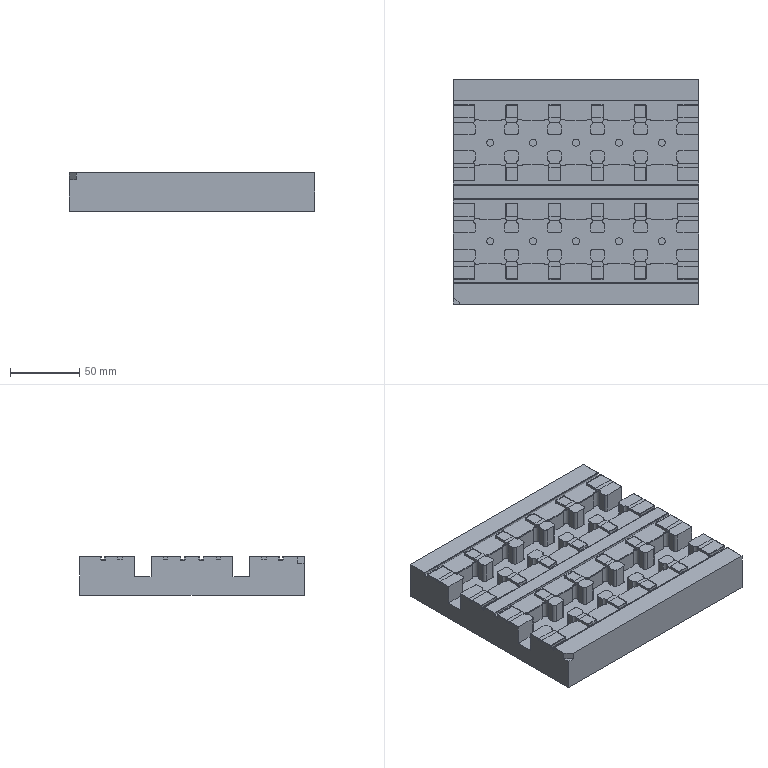NC program | NX | posted by the shop | part box 177 x 162 x 28 mm
Lines 35762 to 36755 of 254847:
N5 T05 M06
(D4  D=4. R=0. H=05 ce=0.02 di=0.05)
(D.N=05 MAX_Z=45. MIN_Z=13.55 Time=46.03M)
T04
G00 G90 G54 X69.164 Y47.661 M03 S4000
G43 H05 Z43.
M08
Z28.502
G01 X69.175 Z28.404 F1200.
X69.205 Y47.665 Z28.317
X69.253 Y47.673 Z28.241
X69.318 Y47.69 Z28.173
X69.396 Y47.717 Z28.114
X69.487 Y47.756 Z28.064
X69.589 Y47.811 Z28.022
X69.699 Y47.883 Z27.987
X69.816 Y47.975 Z27.959
X69.938 Y48.09 Z27.937
X70.063 Y48.229 Z27.921
X70.189 Y48.396 Z27.91
X70.314 Y48.593 Z27.904
X70.437 Y48.822 Z27.902
G02 X71.571 Y49.834 I1.813 J-.891 F1500.
G03 X71.757 Y50.097 I-.094 J.264
X71.663 Y50.307 I-.28 J0.0
G02 X70.986 Y51.668 I1.337 J1.514
G01 X70.965 Y51.832
X70.931 Y51.96 Z27.901
X70.886 Y52.051 Z27.9
X70.83 Y52.11 Z27.899
X70.767 Y52.139 Z27.897
X70.696 Y52.138 Z27.895
X70.62 Y52.112 Z27.893
X70.54 Y52.061 Z27.89
X70.457 Y51.988 Z27.888
X70.374 Y51.896 Z27.885
X70.291 Y51.786 Z27.882
X70.21 Y51.661 Z27.879
X70.132 Y51.523 Z27.875
X70.002 Y51.239 Z27.869
X69.891 Y50.928 Z27.863
X69.801 Y50.597 Z27.856
X69.734 Y50.258 Z27.849
X69.693 Y49.918 Z27.843
X69.678 Y49.588 Z27.837
X69.693 Y49.276 Z27.83
X69.713 Y49.119 Z27.827
X69.742 Y48.973 Z27.824
X69.778 Y48.84 Z27.821
X69.822 Y48.723 Z27.818
X69.872 Y48.625 Z27.815
X69.928 Y48.548 Z27.813
X69.99 Y48.494 Z27.811
X70.056 Y48.467 Z27.809
X70.127 Y48.47 Z27.807
X70.201 Y48.504 Z27.806
X70.277 Y48.572 Z27.805
X70.356 Y48.677 Z27.804
X70.437 Y48.822
G02 X71.571 Y49.834 I1.813 J-.891
G03 X71.757 Y50.097 I-.094 J.264
X71.663 Y50.307 I-.28 J0.0
G02 X70.986 Y51.668 I1.337 J1.514
G01 X70.965 Y51.832 Z27.803
X70.931 Y51.96
X70.886 Y52.051 Z27.802
X70.83 Y52.11 Z27.801
X70.767 Y52.139 Z27.799
X70.696 Y52.138 Z27.797
X70.62 Y52.112 Z27.795
X70.54 Y52.061 Z27.792
X70.457 Y51.988 Z27.789
X70.374 Y51.896 Z27.787
X70.291 Y51.786 Z27.784
X70.21 Y51.661 Z27.78
X70.132 Y51.523 Z27.777
X70.002 Y51.239 Z27.771
X69.891 Y50.928 Z27.764
X69.801 Y50.597 Z27.758
X69.734 Y50.258 Z27.751
X69.693 Y49.918 Z27.745
X69.678 Y49.588 Z27.738
X69.693 Y49.276 Z27.732
X69.713 Y49.119 Z27.729
X69.742 Y48.973 Z27.726
X69.778 Y48.84 Z27.723
X69.822 Y48.723 Z27.72
X69.872 Y48.625 Z27.717
X69.928 Y48.548 Z27.715
X69.99 Y48.494 Z27.712
X70.056 Y48.467 Z27.71
X70.127 Y48.47 Z27.709
X70.201 Y48.504 Z27.707
X70.277 Y48.572 Z27.706
X70.356 Y48.677
X70.437 Y48.822
G02 X71.571 Y49.834 I1.813 J-.891
G03 X71.757 Y50.097 I-.094 J.264
X71.663 Y50.307 I-.28 J0.0
G02 X70.986 Y51.668 I1.337 J1.514
G01 X70.965 Y51.832 Z27.705
X70.931 Y51.96
X70.886 Y52.051 Z27.704
X70.83 Y52.11 Z27.702
X70.767 Y52.139 Z27.701
X70.696 Y52.138 Z27.699
X70.62 Y52.112 Z27.696
X70.54 Y52.061 Z27.694
X70.457 Y51.988 Z27.691
X70.374 Y51.896 Z27.688
X70.291 Y51.786 Z27.685
X70.21 Y51.661 Z27.682
X70.132 Y51.523 Z27.679
X70.002 Y51.239 Z27.673
X69.891 Y50.928 Z27.666
X69.801 Y50.597 Z27.66
X69.734 Y50.258 Z27.653
X69.693 Y49.918 Z27.647
X69.678 Y49.588 Z27.64
X69.693 Y49.276 Z27.634
X69.713 Y49.119 Z27.631
X69.742 Y48.973 Z27.628
X69.778 Y48.84 Z27.625
X69.822 Y48.723 Z27.622
X69.872 Y48.625 Z27.619
X69.928 Y48.548 Z27.616
X69.99 Y48.494 Z27.614
X70.056 Y48.467 Z27.612
X70.127 Y48.47 Z27.611
X70.201 Y48.504 Z27.609
X70.277 Y48.572 Z27.608
X70.356 Y48.677
X70.437 Y48.822 Z27.607
G02 X71.571 Y49.834 I1.813 J-.891
G03 X71.757 Y50.097 I-.094 J.264
X71.663 Y50.307 I-.28 J0.0
G02 X70.986 Y51.668 I1.337 J1.514
G01 X70.965 Y51.832
X70.931 Y51.96
X70.886 Y52.051 Z27.606
X70.83 Y52.11 Z27.604
X70.767 Y52.139 Z27.603
X70.696 Y52.138 Z27.601
X70.62 Y52.112 Z27.598
X70.54 Y52.061 Z27.596
X70.457 Y51.988 Z27.593
X70.374 Y51.896 Z27.59
X70.291 Y51.786 Z27.587
X70.21 Y51.661 Z27.584
X70.132 Y51.523 Z27.581
X70.002 Y51.239 Z27.575
X69.891 Y50.928 Z27.568
X69.801 Y50.597 Z27.562
X69.734 Y50.258 Z27.555
X69.693 Y49.918 Z27.549
X69.678 Y49.588 Z27.542
X69.693 Y49.276 Z27.536
X69.713 Y49.119 Z27.533
X69.742 Y48.973 Z27.529
X69.778 Y48.84 Z27.526
X69.822 Y48.723 Z27.524
X69.872 Y48.625 Z27.521
X69.928 Y48.548 Z27.518
X69.99 Y48.494 Z27.516
X70.056 Y48.467 Z27.514
X70.127 Y48.47 Z27.512
X70.201 Y48.504 Z27.511
X70.277 Y48.572 Z27.51
X70.356 Y48.677 Z27.509
X70.437 Y48.822
G02 X71.571 Y49.834 I1.813 J-.891
G03 X71.757 Y50.097 I-.094 J.264
X71.663 Y50.307 I-.28 J0.0
G02 X70.986 Y51.668 I1.337 J1.514
G01 X70.965 Y51.832
X70.931 Y51.96 Z27.508
X70.886 Y52.051 Z27.507
X70.83 Y52.11 Z27.506
X70.767 Y52.139 Z27.504
X70.696 Y52.138 Z27.502
X70.62 Y52.112 Z27.5
X70.54 Y52.061 Z27.498
X70.457 Y51.988 Z27.495
X70.374 Y51.896 Z27.492
X70.291 Y51.786 Z27.489
X70.21 Y51.661 Z27.486
X70.132 Y51.523 Z27.483
X70.002 Y51.239 Z27.476
X69.891 Y50.928 Z27.47
X69.801 Y50.597 Z27.463
X69.734 Y50.258 Z27.457
X69.693 Y49.918 Z27.45
X69.678 Y49.588 Z27.444
X69.693 Y49.276 Z27.438
X69.713 Y49.119 Z27.434
X69.742 Y48.973 Z27.431
X69.778 Y48.84 Z27.428
X69.822 Y48.723 Z27.425
X69.872 Y48.625 Z27.423
X69.928 Y48.548 Z27.42
X69.99 Y48.494 Z27.418
X70.056 Y48.467 Z27.416
X70.127 Y48.47 Z27.414
X70.201 Y48.504 Z27.413
X70.277 Y48.572 Z27.412
X70.356 Y48.677 Z27.411
X70.437 Y48.822
G02 X71.571 Y49.834 I1.813 J-.891
G03 X71.757 Y50.097 I-.094 J.264
X71.663 Y50.307 I-.28 J0.0
G02 X70.986 Y51.668 I1.337 J1.514
G01 X70.965 Y51.832
X70.931 Y51.96 Z27.41
X70.886 Y52.051 Z27.409
X70.83 Y52.11 Z27.408
X70.767 Y52.139 Z27.406
X70.696 Y52.138 Z27.404
X70.62 Y52.112 Z27.402
X70.54 Y52.061 Z27.4
X70.457 Y51.988 Z27.397
X70.374 Y51.896 Z27.394
X70.291 Y51.786 Z27.391
X70.21 Y51.661 Z27.388
X70.132 Y51.523 Z27.385
X70.002 Y51.239 Z27.378
X69.891 Y50.928 Z27.372
X69.801 Y50.597 Z27.365
X69.734 Y50.258 Z27.359
X69.693 Y49.918 Z27.352
X69.678 Y49.588 Z27.346
X69.693 Y49.276 Z27.34
X69.713 Y49.119 Z27.336
X69.742 Y48.973 Z27.333
X69.778 Y48.84 Z27.33
X69.822 Y48.723 Z27.327
X69.872 Y48.625 Z27.325
X69.928 Y48.548 Z27.322
X69.99 Y48.494 Z27.32
X70.056 Y48.467 Z27.318
X70.127 Y48.47 Z27.316
X70.201 Y48.504 Z27.315
X70.277 Y48.572 Z27.314
X70.356 Y48.677 Z27.313
X70.437 Y48.822
G02 X71.571 Y49.834 I1.813 J-.891
G03 X71.757 Y50.097 I-.094 J.264
X71.663 Y50.307 I-.28 J0.0
G02 X70.986 Y51.668 I1.337 J1.514
G01 X70.965 Y51.832
X70.931 Y51.96 Z27.312
X70.886 Y52.051 Z27.311
X70.83 Y52.11 Z27.31
X70.767 Y52.139 Z27.308
X70.696 Y52.138 Z27.306
X70.62 Y52.112 Z27.304
X70.54 Y52.061 Z27.301
X70.457 Y51.988 Z27.299
X70.374 Y51.896 Z27.296
X70.291 Y51.786 Z27.293
X70.21 Y51.661 Z27.29
X70.132 Y51.523 Z27.286
X70.002 Y51.239 Z27.28
X69.891 Y50.928 Z27.274
X69.801 Y50.597 Z27.267
X69.734 Y50.258 Z27.261
X69.693 Y49.918 Z27.254
X69.678 Y49.588 Z27.248
X69.693 Y49.276 Z27.241
X69.713 Y49.119 Z27.238
X69.742 Y48.973 Z27.235
X69.778 Y48.84 Z27.232
X69.822 Y48.723 Z27.229
X69.872 Y48.625 Z27.226
X69.928 Y48.548 Z27.224
X69.99 Y48.494 Z27.222
X70.056 Y48.467 Z27.22
X70.127 Y48.47 Z27.218
X70.201 Y48.504 Z27.217
X70.277 Y48.572 Z27.216
X70.356 Y48.677 Z27.215
X70.437 Y48.822
G02 X71.571 Y49.834 I1.813 J-.891
G03 X71.757 Y50.097 I-.094 J.264
X71.663 Y50.307 I-.28 J0.0
G02 X70.986 Y51.668 I1.337 J1.514
G01 X70.965 Y51.832
X70.931 Y51.96 Z27.214
X70.886 Y52.051 Z27.213
X70.83 Y52.11 Z27.212
X70.767 Y52.139 Z27.21
X70.696 Y52.138 Z27.208
X70.62 Y52.112 Z27.206
X70.54 Y52.061 Z27.203
X70.457 Y51.988 Z27.201
X70.374 Y51.896 Z27.198
X70.291 Y51.786 Z27.195
X70.21 Y51.661 Z27.191
X70.132 Y51.523 Z27.188
X70.002 Y51.239 Z27.182
X69.891 Y50.928 Z27.176
X69.801 Y50.597 Z27.169
X69.734 Y50.258 Z27.162
X69.693 Y49.918 Z27.156
X69.678 Y49.588 Z27.149
X69.693 Y49.276 Z27.143
X69.713 Y49.119 Z27.14
X69.742 Y48.973 Z27.137
X69.778 Y48.84 Z27.134
X69.822 Y48.723 Z27.131
X69.872 Y48.625 Z27.128
X69.928 Y48.548 Z27.126
X69.99 Y48.494 Z27.124
X70.056 Y48.467 Z27.122
X70.127 Y48.47 Z27.12
X70.201 Y48.504 Z27.119
X70.277 Y48.572 Z27.118
X70.356 Y48.677 Z27.117
X70.437 Y48.822
G02 X71.571 Y49.834 I1.813 J-.891
G03 X71.757 Y50.097 I-.094 J.264
X71.663 Y50.307 I-.28 J0.0
G02 X70.986 Y51.668 I1.337 J1.514
G01 X70.965 Y51.832 Z27.116
X70.931 Y51.96
X70.886 Y52.051 Z27.115
X70.83 Y52.11 Z27.113
X70.767 Y52.139 Z27.112
X70.696 Y52.138 Z27.11
X70.62 Y52.112 Z27.108
X70.54 Y52.061 Z27.105
X70.457 Y51.988 Z27.102
X70.374 Y51.896 Z27.1
X70.291 Y51.786 Z27.097
X70.21 Y51.661 Z27.093
X70.132 Y51.523 Z27.09
X70.002 Y51.239 Z27.084
X69.891 Y50.928 Z27.077
X69.801 Y50.597 Z27.071
X69.734 Y50.258 Z27.064
X69.693 Y49.918 Z27.058
X69.678 Y49.588 Z27.051
X69.693 Y49.276 Z27.045
X69.713 Y49.119 Z27.042
X69.742 Y48.973 Z27.039
X69.778 Y48.84 Z27.036
X69.822 Y48.723 Z27.033
X69.872 Y48.625 Z27.03
X69.928 Y48.548 Z27.028
X69.99 Y48.494 Z27.025
X70.056 Y48.467 Z27.023
X70.127 Y48.47 Z27.022
X70.201 Y48.504 Z27.02
X70.277 Y48.572 Z27.019
X70.356 Y48.677
X70.437 Y48.822
G02 X71.571 Y49.834 I1.813 J-.891
G03 X71.757 Y50.097 I-.094 J.264
X71.663 Y50.307 I-.28 J0.0
G02 X70.986 Y51.668 I1.337 J1.514
G01 X70.965 Y51.832 Z27.018
X70.931 Y51.96
X70.886 Y52.051 Z27.017
X70.83 Y52.11 Z27.015
X70.767 Y52.139 Z27.014
X70.696 Y52.138 Z27.012
X70.62 Y52.112 Z27.009
X70.54 Y52.061 Z27.007
X70.457 Y51.988 Z27.004
X70.374 Y51.896 Z27.001
X70.291 Y51.786 Z26.998
X70.21 Y51.661 Z26.995
X70.132 Y51.523 Z26.992
X70.002 Y51.239 Z26.986
X69.891 Y50.928 Z26.979
X69.801 Y50.597 Z26.973
X69.734 Y50.258 Z26.966
X69.693 Y49.918 Z26.96
X69.678 Y49.588 Z26.953
X69.693 Y49.276 Z26.947
X69.713 Y49.119 Z26.944
X69.742 Y48.973 Z26.941
X69.778 Y48.84 Z26.937
X69.822 Y48.723 Z26.935
X69.872 Y48.625 Z26.932
X69.928 Y48.548 Z26.929
X69.99 Y48.494 Z26.927
X70.056 Y48.467 Z26.925
X70.127 Y48.47 Z26.924
X70.201 Y48.504 Z26.922
X70.277 Y48.572 Z26.921
X70.356 Y48.677
X70.437 Y48.822 Z26.92
G02 X71.571 Y49.834 I1.813 J-.891
G03 X71.757 Y50.097 I-.094 J.264
X71.663 Y50.307 I-.28 J0.0
G02 X70.986 Y51.668 I1.337 J1.514
G01 X70.965 Y51.832
X70.931 Y51.96
X70.886 Y52.051 Z26.919
X70.83 Y52.11 Z26.917
X70.767 Y52.139 Z26.916
X70.696 Y52.138 Z26.914
X70.62 Y52.112 Z26.911
X70.54 Y52.061 Z26.909
X70.457 Y51.988 Z26.906
X70.374 Y51.896 Z26.903
X70.291 Y51.786 Z26.9
X70.21 Y51.661 Z26.897
X70.132 Y51.523 Z26.894
X70.002 Y51.239 Z26.888
X69.891 Y50.928 Z26.881
X69.801 Y50.597 Z26.875
X69.734 Y50.258 Z26.868
X69.693 Y49.918 Z26.861
X69.678 Y49.588 Z26.855
X69.693 Y49.276 Z26.849
X69.713 Y49.119 Z26.846
X69.742 Y48.973 Z26.842
X69.778 Y48.84 Z26.839
X69.822 Y48.723 Z26.836
X69.872 Y48.625 Z26.834
X69.928 Y48.548 Z26.831
X69.99 Y48.494 Z26.829
X70.056 Y48.467 Z26.827
X70.127 Y48.47 Z26.825
X70.201 Y48.504 Z26.824
X70.277 Y48.572 Z26.823
X70.356 Y48.677 Z26.822
X70.437 Y48.822
G02 X71.571 Y49.834 I1.813 J-.891
G03 X71.757 Y50.097 I-.094 J.264
X71.663 Y50.307 I-.28 J0.0
G02 X70.986 Y51.668 I1.337 J1.514
G01 X70.965 Y51.832
X70.931 Y51.96 Z26.821
X70.886 Y52.051 Z26.82
X70.83 Y52.11 Z26.819
X70.767 Y52.139 Z26.817
X70.696 Y52.138 Z26.815
X70.62 Y52.112 Z26.813
X70.54 Y52.061 Z26.811
X70.457 Y51.988 Z26.808
X70.374 Y51.896 Z26.805
X70.291 Y51.786 Z26.802
X70.21 Y51.661 Z26.799
X70.132 Y51.523 Z26.796
X70.002 Y51.239 Z26.789
X69.891 Y50.928 Z26.783
X69.801 Y50.597 Z26.776
X69.734 Y50.258 Z26.77
X69.693 Y49.918 Z26.763
X69.678 Y49.588 Z26.757
X69.693 Y49.276 Z26.751
X69.713 Y49.119 Z26.747
X69.742 Y48.973 Z26.744
X69.778 Y48.84 Z26.741
X69.822 Y48.723 Z26.738
X69.872 Y48.625 Z26.736
X69.928 Y48.548 Z26.733
X69.99 Y48.494 Z26.731
X70.056 Y48.467 Z26.729
X70.127 Y48.47 Z26.727
X70.201 Y48.504 Z26.726
X70.277 Y48.572 Z26.725
X70.356 Y48.677 Z26.724
X70.437 Y48.822
G02 X71.571 Y49.834 I1.813 J-.891
G03 X71.757 Y50.097 I-.094 J.264
X71.663 Y50.307 I-.28 J0.0
G02 X70.986 Y51.668 I1.337 J1.514
G01 X70.965 Y51.832
X70.931 Y51.96 Z26.723
X70.886 Y52.051 Z26.722
X70.83 Y52.11 Z26.721
X70.767 Y52.139 Z26.719
X70.696 Y52.138 Z26.717
X70.62 Y52.112 Z26.715
X70.54 Y52.061 Z26.713
X70.457 Y51.988 Z26.71
X70.374 Y51.896 Z26.707
X70.291 Y51.786 Z26.704
X70.21 Y51.661 Z26.701
X70.132 Y51.523 Z26.697
X70.002 Y51.239 Z26.691
X69.891 Y50.928 Z26.685
X69.801 Y50.597 Z26.678
X69.734 Y50.258 Z26.672
X69.693 Y49.918 Z26.665
X69.678 Y49.588 Z26.659
X69.693 Y49.276 Z26.653
X69.713 Y49.119 Z26.649
X69.742 Y48.973 Z26.646
X69.778 Y48.84 Z26.643
X69.822 Y48.723 Z26.64
X69.872 Y48.625 Z26.637
X69.928 Y48.548 Z26.635
X69.99 Y48.494 Z26.633
X70.056 Y48.467 Z26.631
X70.127 Y48.47 Z26.629
X70.201 Y48.504 Z26.628
X70.277 Y48.572 Z26.627
X70.356 Y48.677 Z26.626
X70.437 Y48.822
G02 X71.571 Y49.834 I1.813 J-.891
G03 X71.757 Y50.097 I-.094 J.264
X71.663 Y50.307 I-.28 J0.0
G02 X70.986 Y51.668 I1.337 J1.514
G01 X70.965 Y51.832
X70.931 Y51.96 Z26.625
X70.886 Y52.051 Z26.624
X70.83 Y52.11 Z26.623
X70.767 Y52.139 Z26.621
X70.696 Y52.138 Z26.619
X70.62 Y52.112 Z26.617
X70.54 Y52.061 Z26.614
X70.457 Y51.988 Z26.612
X70.374 Y51.896 Z26.609
X70.291 Y51.786 Z26.606
X70.21 Y51.661 Z26.603
X70.132 Y51.523 Z26.599
X70.002 Y51.239 Z26.593
X69.891 Y50.928 Z26.587
X69.801 Y50.597 Z26.58
X69.734 Y50.258 Z26.574
X69.693 Y49.918 Z26.567
X69.678 Y49.588 Z26.561
X69.693 Y49.276 Z26.554
X69.713 Y49.119 Z26.551
X69.742 Y48.973 Z26.548
X69.778 Y48.84 Z26.545
X69.822 Y48.723 Z26.542
X69.872 Y48.625 Z26.539
X69.928 Y48.548 Z26.537
X69.99 Y48.494 Z26.535
X70.056 Y48.467 Z26.533
X70.127 Y48.47 Z26.531
X70.201 Y48.504 Z26.53
X70.277 Y48.572 Z26.529
X70.356 Y48.677 Z26.528
X70.437 Y48.822
G02 X71.571 Y49.834 I1.813 J-.891
G03 X71.757 Y50.097 I-.094 J.264
X71.663 Y50.307 I-.28 J0.0
G02 X70.986 Y51.668 I1.337 J1.514
G01 X70.965 Y51.832
X70.931 Y51.96 Z26.527
X70.886 Y52.051 Z26.526
X70.83 Y52.11 Z26.525
X70.767 Y52.139 Z26.523
X70.696 Y52.138 Z26.521
X70.62 Y52.112 Z26.519
X70.54 Y52.061 Z26.516
X70.457 Y51.988 Z26.514
X70.374 Y51.896 Z26.511
X70.291 Y51.786 Z26.508
X70.21 Y51.661 Z26.504
X70.132 Y51.523 Z26.501
X70.002 Y51.239 Z26.495
X69.891 Y50.928 Z26.489
X69.801 Y50.597 Z26.482
X69.734 Y50.258 Z26.475
X69.693 Y49.918 Z26.469
X69.678 Y49.588 Z26.462
X69.693 Y49.276 Z26.456
X69.713 Y49.119 Z26.453
X69.742 Y48.973 Z26.45
X69.778 Y48.84 Z26.447
X69.822 Y48.723 Z26.444
X69.872 Y48.625 Z26.441
X69.928 Y48.548 Z26.439
X69.99 Y48.494 Z26.436
X70.056 Y48.467 Z26.434
X70.127 Y48.47 Z26.433
X70.201 Y48.504 Z26.431
X70.277 Y48.572 Z26.43
X70.356 Y48.677
X70.437 Y48.822
G02 X71.571 Y49.834 I1.813 J-.891
G03 X71.757 Y50.097 I-.094 J.264
X71.663 Y50.307 I-.28 J0.0
G02 X70.986 Y51.668 I1.337 J1.514
G01 X70.965 Y51.832 Z26.429
X70.931 Y51.96
X70.886 Y52.051 Z26.428
X70.83 Y52.11 Z26.426
X70.767 Y52.139 Z26.425
X70.696 Y52.138 Z26.423
X70.62 Y52.112 Z26.421
X70.54 Y52.061 Z26.418
X70.457 Y51.988 Z26.415
X70.374 Y51.896 Z26.413
X70.291 Y51.786 Z26.409
X70.21 Y51.661 Z26.406
X70.132 Y51.523 Z26.403
X70.002 Y51.239 Z26.397
X69.891 Y50.928 Z26.39
X69.801 Y50.597 Z26.384
X69.734 Y50.258 Z26.377
X69.693 Y49.918 Z26.371
X69.678 Y49.588 Z26.364
X69.693 Y49.276 Z26.358
X69.713 Y49.119 Z26.355
X69.742 Y48.973 Z26.352
X69.778 Y48.84 Z26.349
X69.822 Y48.723 Z26.346
X69.872 Y48.625 Z26.343
X69.928 Y48.548 Z26.341
X69.99 Y48.494 Z26.338
X70.056 Y48.467 Z26.336
X70.127 Y48.47 Z26.335
X70.201 Y48.504 Z26.333
X70.277 Y48.572 Z26.332
X70.356 Y48.677
X70.437 Y48.822 Z26.331
G02 X71.571 Y49.834 I1.813 J-.891
G03 X71.757 Y50.097 I-.094 J.264
X71.663 Y50.307 I-.28 J0.0
G02 X70.986 Y51.668 I1.337 J1.514
G01 X70.965 Y51.832
X70.931 Y51.96
X70.886 Y52.051 Z26.33
X70.83 Y52.11 Z26.328
X70.767 Y52.139 Z26.327
X70.696 Y52.138 Z26.325
X70.62 Y52.112 Z26.322
X70.54 Y52.061 Z26.32
X70.457 Y51.988 Z26.317
X70.374 Y51.896 Z26.314
X70.291 Y51.786 Z26.311
X70.21 Y51.661 Z26.308
X70.132 Y51.523 Z26.305
X70.002 Y51.239 Z26.299
X69.891 Y50.928 Z26.292
X69.801 Y50.597 Z26.286
X69.734 Y50.258 Z26.279
X69.693 Y49.918 Z26.273
X69.678 Y49.588 Z26.266
X69.693 Y49.276 Z26.26
X69.713 Y49.119 Z26.257
X69.742 Y48.973 Z26.253
X69.778 Y48.84 Z26.25
X69.822 Y48.723 Z26.248
X69.872 Y48.625 Z26.245
X69.928 Y48.548 Z26.242
X69.99 Y48.494 Z26.24
X70.056 Y48.467 Z26.238
X70.127 Y48.47 Z26.237
X70.201 Y48.504 Z26.235
X70.277 Y48.572 Z26.234
X70.356 Y48.677
X70.437 Y48.822 Z26.233
G02 X71.571 Y49.834 I1.813 J-.891
G03 X71.757 Y50.097 I-.094 J.264
X71.663 Y50.307 I-.28 J0.0
G02 X70.986 Y51.668 I1.337 J1.514
G01 X70.965 Y51.832
X70.931 Y51.96
X70.886 Y52.051 Z26.231
X70.83 Y52.11 Z26.23
X70.767 Y52.139 Z26.228
X70.696 Y52.138 Z26.226
X70.62 Y52.112 Z26.224
X70.54 Y52.061 Z26.222
X70.457 Y51.988 Z26.219
X70.374 Y51.896 Z26.216
X70.291 Y51.786 Z26.213
X70.21 Y51.661 Z26.21
X70.132 Y51.523 Z26.207
X70.002 Y51.239 Z26.201
X69.891 Y50.928 Z26.194
X69.801 Y50.597 Z26.188
X69.734 Y50.258 Z26.181
X69.693 Y49.918 Z26.174
X69.678 Y49.588 Z26.168
X69.693 Y49.276 Z26.162
X69.713 Y49.119 Z26.159
X69.742 Y48.973 Z26.155
X69.778 Y48.84 Z26.152
X69.822 Y48.723 Z26.149
X69.872 Y48.625 Z26.147
X69.928 Y48.548 Z26.144
X69.99 Y48.494 Z26.142
X70.056 Y48.467 Z26.14
X70.127 Y48.47 Z26.138
X70.201 Y48.504 Z26.137
X70.277 Y48.572 Z26.136
X70.356 Y48.677 Z26.135
X70.437 Y48.822
G02 X71.571 Y49.834 I1.813 J-.891
G03 X71.757 Y50.097 I-.094 J.264
X71.663 Y50.307 I-.28 J0.0
G02 X70.986 Y51.668 I1.337 J1.514
G01 X70.965 Y51.832
X70.931 Y51.96 Z26.134
X70.886 Y52.051 Z26.133
X70.83 Y52.11 Z26.132
X70.767 Y52.139 Z26.13
X70.696 Y52.138 Z26.128
X70.62 Y52.112 Z26.126
X70.54 Y52.061 Z26.124
X70.457 Y51.988 Z26.121
X70.374 Y51.896 Z26.118
X70.291 Y51.786 Z26.115
X70.21 Y51.661 Z26.112
X70.132 Y51.523 Z26.109
X70.002 Y51.239 Z26.102
X69.891 Y50.928 Z26.096
X69.801 Y50.597 Z26.089
X69.734 Y50.258 Z26.083
X69.693 Y49.918 Z26.076
X69.678 Y49.588 Z26.07
X69.693 Y49.276 Z26.064
X69.713 Y49.119 Z26.06
X69.742 Y48.973 Z26.057
X69.778 Y48.84 Z26.054
X69.822 Y48.723 Z26.051
X69.872 Y48.625 Z26.049
X69.928 Y48.548 Z26.046
X69.99 Y48.494 Z26.044
X70.056 Y48.467 Z26.042
X70.127 Y48.47 Z26.04
X70.201 Y48.504 Z26.039
X70.277 Y48.572 Z26.038
X70.356 Y48.677 Z26.037
X70.437 Y48.822
G02 X71.571 Y49.834 I1.813 J-.891
G03 X71.757 Y50.097 I-.094 J.264
X71.663 Y50.307 I-.28 J0.0
G02 X70.986 Y51.668 I1.337 J1.514
G01 X70.965 Y51.832
X70.931 Y51.96 Z26.036
X70.886 Y52.051 Z26.035
X70.83 Y52.11 Z26.034
X70.767 Y52.139 Z26.032
X70.696 Y52.138 Z26.03
X70.62 Y52.112 Z26.028
X70.54 Y52.061 Z26.025
X70.457 Y51.988 Z26.023
X70.374 Y51.896 Z26.02
X70.291 Y51.786 Z26.017
X70.21 Y51.661 Z26.014
X70.132 Y51.523 Z26.01
X70.002 Y51.239 Z26.004
X69.891 Y50.928 Z25.998
X69.801 Y50.597 Z25.991
X69.734 Y50.258 Z25.985
X69.693 Y49.918 Z25.978
X69.678 Y49.588 Z25.972
X69.693 Y49.276 Z25.965
X69.713 Y49.119 Z25.962
X69.742 Y48.973 Z25.959
X69.778 Y48.84 Z25.956
X69.822 Y48.723 Z25.953
X69.872 Y48.625 Z25.95
X69.928 Y48.548 Z25.948
X69.99 Y48.494 Z25.946
X70.056 Y48.467 Z25.944
X70.127 Y48.47 Z25.942
X70.201 Y48.504 Z25.941
X70.277 Y48.572 Z25.94
X70.356 Y48.677 Z25.939
X70.437 Y48.822
G02 X71.571 Y49.834 I1.813 J-.891
G03 X71.757 Y50.097 I-.094 J.264
X71.663 Y50.307 I-.28 J0.0
G02 X70.986 Y51.668 I1.337 J1.514
G01 X70.965 Y51.832
X70.931 Y51.96 Z25.938
X70.886 Y52.051 Z25.937
X70.83 Y52.11 Z25.936
X70.767 Y52.139 Z25.934
X70.696 Y52.138 Z25.932
X70.62 Y52.112 Z25.93
X70.54 Y52.061 Z25.927
X70.457 Y51.988 Z25.925
X70.374 Y51.896 Z25.922
X70.291 Y51.786 Z25.919
X70.21 Y51.661 Z25.916
X70.132 Y51.523 Z25.912
X70.002 Y51.239 Z25.906
X69.891 Y50.928 Z25.9
X69.801 Y50.597 Z25.893
X69.734 Y50.258 Z25.887
X69.693 Y49.918 Z25.88
X69.678 Y49.588 Z25.874
X69.693 Y49.276 Z25.867
X69.713 Y49.119 Z25.864
X69.742 Y48.973 Z25.861
X69.778 Y48.84 Z25.858
X69.822 Y48.723 Z25.855
X69.872 Y48.625 Z25.852
X69.928 Y48.548 Z25.85
X69.99 Y48.494 Z25.848
X70.056 Y48.467 Z25.846
X70.127 Y48.47 Z25.844
X70.201 Y48.504 Z25.843
X70.277 Y48.572 Z25.842
X70.356 Y48.677 Z25.841
X70.437 Y48.822
G02 X71.571 Y49.834 I1.813 J-.891
G03 X71.757 Y50.097 I-.094 J.264
X71.663 Y50.307 I-.28 J0.0
G02 X70.986 Y51.668 I1.337 J1.514
G01 X70.965 Y51.832
X70.931 Y51.96 Z25.84
X70.886 Y52.051 Z25.839
X70.83 Y52.11 Z25.838
X70.767 Y52.139 Z25.836
X70.696 Y52.138 Z25.834
X70.62 Y52.112 Z25.832
X70.54 Y52.061 Z25.829
X70.457 Y51.988 Z25.826
X70.374 Y51.896 Z25.824
X70.291 Y51.786 Z25.821
X70.21 Y51.661 Z25.817
X70.132 Y51.523 Z25.814
X70.002 Y51.239 Z25.808
X69.891 Y50.928 Z25.801
X69.801 Y50.597 Z25.795
X69.734 Y50.258 Z25.788
X69.693 Y49.918 Z25.782
X69.678 Y49.588 Z25.775
X69.693 Y49.276 Z25.769
X69.713 Y49.119 Z25.766
X69.742 Y48.973 Z25.763
X69.778 Y48.84 Z25.76
X69.822 Y48.723 Z25.757
X69.872 Y48.625 Z25.754
X69.928 Y48.548 Z25.752
X69.99 Y48.494 Z25.749
X70.056 Y48.467 Z25.747
X70.127 Y48.47 Z25.746
X70.201 Y48.504 Z25.744
X70.277 Y48.572 Z25.743
X70.356 Y48.677
X70.437 Y48.822
G02 X71.571 Y49.834 I1.813 J-.891
G03 X71.757 Y50.097 I-.094 J.264
X71.663 Y50.307 I-.28 J0.0
G02 X70.986 Y51.668 I1.337 J1.514
G01 X70.965 Y51.832 Z25.742
X70.931 Y51.96
X70.886 Y52.051 Z25.741
X70.83 Y52.11 Z25.739
X70.767 Y52.139 Z25.738
X70.696 Y52.138 Z25.736
X70.62 Y52.112 Z25.734
X70.54 Y52.061 Z25.731
X70.457 Y51.988 Z25.728
X70.374 Y51.896 Z25.725
X70.291 Y51.786 Z25.722
X70.21 Y51.661 Z25.719
X70.132 Y51.523 Z25.716
X70.002 Y51.239 Z25.71
X69.891 Y50.928 Z25.703
X69.801 Y50.597 Z25.697
X69.734 Y50.258 Z25.69
X69.693 Y49.918 Z25.684
X69.678 Y49.588 Z25.677
X69.693 Y49.276 Z25.671
X69.713 Y49.119 Z25.668
X69.742 Y48.973 Z25.665
X69.778 Y48.84 Z25.662
X69.822 Y48.723 Z25.659
X69.872 Y48.625 Z25.656
X69.928 Y48.548 Z25.654
X69.99 Y48.494 Z25.651
X70.056 Y48.467 Z25.649
X70.127 Y48.47 Z25.648
X70.201 Y48.504 Z25.646
X70.277 Y48.572 Z25.645
X70.356 Y48.677
X70.437 Y48.822 Z25.644
G02 X71.571 Y49.834 I1.813 J-.891
G03 X71.757 Y50.097 I-.094 J.264
X71.663 Y50.307 I-.28 J0.0
G02 X70.986 Y51.668 I1.337 J1.514
G01 X70.965 Y51.832
X70.931 Y51.96
X70.886 Y52.051 Z25.643
X70.83 Y52.11 Z25.641
X70.767 Y52.139 Z25.64
X70.696 Y52.138 Z25.638
X70.62 Y52.112 Z25.635
X70.54 Y52.061 Z25.633
X70.457 Y51.988 Z25.63
X70.374 Y51.896 Z25.627
X70.291 Y51.786 Z25.624
X70.21 Y51.661 Z25.621
X70.132 Y51.523 Z25.618
X70.002 Y51.239 Z25.612
X69.891 Y50.928 Z25.605
X69.801 Y50.597 Z25.599
X69.734 Y50.258 Z25.592
X69.693 Y49.918 Z25.586
X69.678 Y49.588 Z25.579
X69.693 Y49.276 Z25.573
X69.713 Y49.119 Z25.57
X69.742 Y48.973 Z25.566
X69.778 Y48.84 Z25.563
X69.822 Y48.723 Z25.561
X69.872 Y48.625 Z25.558
X69.928 Y48.548 Z25.555
X69.99 Y48.494 Z25.553
X70.056 Y48.467 Z25.551
X70.127 Y48.47 Z25.549
X70.201 Y48.504 Z25.548
X70.277 Y48.572 Z25.547
X70.356 Y48.677
X70.437 Y48.822 Z25.546
G02 X71.571 Y49.834 I1.813 J-.891
G03 X71.757 Y50.097 I-.094 J.264
X71.663 Y50.307 I-.28 J0.0
G02 X70.986 Y51.668 I1.337 J1.514
G01 X70.965 Y51.832
X70.931 Y51.96 Z25.545
X70.886 Y52.051 Z25.544
X70.83 Y52.11 Z25.543
X70.767 Y52.139 Z25.541
X70.696 Y52.138 Z25.539
X70.62 Y52.112 Z25.537
X70.54 Y52.061 Z25.535
X70.457 Y51.988 Z25.532
X70.374 Y51.896 Z25.529
X70.291 Y51.786 Z25.526
X70.21 Y51.661 Z25.523
X70.132 Y51.523 Z25.52
X70.002 Y51.239 Z25.513
X69.891 Y50.928 Z25.507
X69.801 Y50.597 Z25.501
X69.734 Y50.258 Z25.494
X69.693 Y49.918 Z25.487
X69.678 Y49.588 Z25.481
X69.693 Y49.276 Z25.475
X69.713 Y49.119 Z25.471
X69.742 Y48.973 Z25.468
X69.778 Y48.84 Z25.465
X69.822 Y48.723 Z25.462
X69.872 Y48.625 Z25.46
X69.928 Y48.548 Z25.457
X69.99 Y48.494 Z25.455
X70.056 Y48.467 Z25.453
X70.127 Y48.47 Z25.451
X70.201 Y48.504 Z25.45
X70.277 Y48.572 Z25.449
X70.356 Y48.677 Z25.448
X70.437 Y48.822
G02 X71.571 Y49.834 I1.813 J-.891
G03 X71.757 Y50.097 I-.094 J.264
X71.663 Y50.307 I-.28 J0.0
G02 X70.986 Y51.668 I1.337 J1.514
G01 X70.965 Y51.832
X70.931 Y51.96 Z25.447
X70.886 Y52.051 Z25.446
X70.83 Y52.11 Z25.445
X70.767 Y52.139 Z25.443
X70.696 Y52.138 Z25.441
X70.62 Y52.112 Z25.439
X70.54 Y52.061 Z25.437
X70.457 Y51.988 Z25.434
X70.374 Y51.896 Z25.431
X70.291 Y51.786 Z25.428
X70.21 Y51.661 Z25.425
X70.132 Y51.523 Z25.422
X70.002 Y51.239 Z25.415
X69.891 Y50.928 Z25.409
X69.801 Y50.597 Z25.402
X69.734 Y50.258 Z25.396
X69.693 Y49.918 Z25.389
X69.678 Y49.588 Z25.383
X69.693 Y49.276 Z25.377
X69.713 Y49.119 Z25.373
X69.742 Y48.973 Z25.37
X69.778 Y48.84 Z25.367
X69.822 Y48.723 Z25.364
X69.872 Y48.625 Z25.362
X69.928 Y48.548 Z25.359
X69.99 Y48.494 Z25.357
X70.056 Y48.467 Z25.355
X70.127 Y48.47 Z25.353
X70.201 Y48.504 Z25.352
X70.277 Y48.572 Z25.351
X70.356 Y48.677 Z25.35
X70.437 Y48.822
G02 X71.571 Y49.834 I1.813 J-.891
G03 X71.757 Y50.097 I-.094 J.264
X71.663 Y50.307 I-.28 J0.0
G02 X70.986 Y51.668 I1.337 J1.514
G01 X70.957 Y51.944 Z25.361
X70.912 Y52.239 Z25.394
X70.856 Y52.549 Z25.446
X70.791 Y52.872 Z25.516
X70.656 Y53.517 Z25.691
X70.575 Y53.925 Z25.818